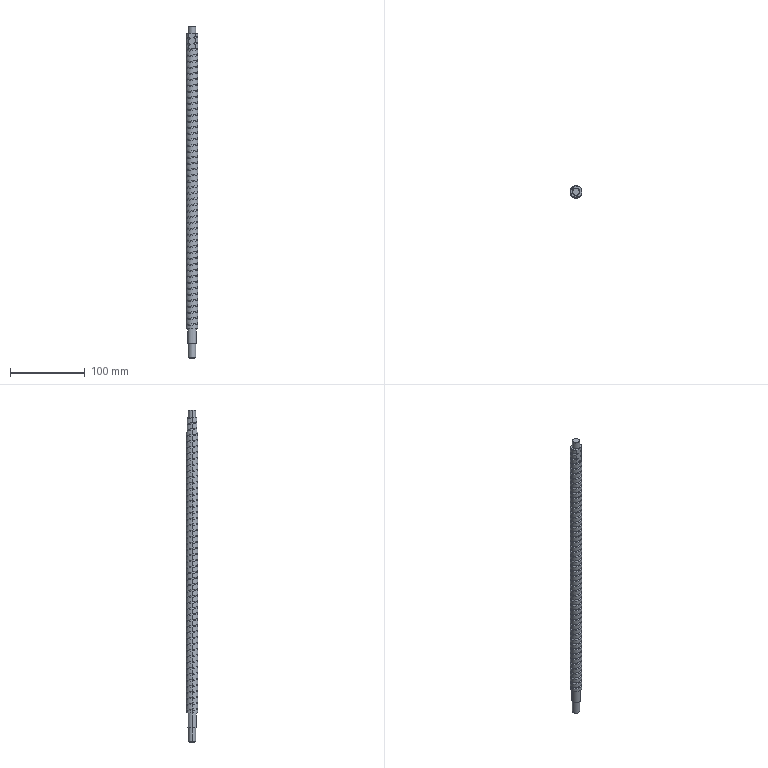Part | STEP file | Ball screw assembly SFUR1604-445 | 1 solid | 136 faces | box 16 x 16 x 445 mm | volume 80049 mm3 | cylinder 114 | plane 12 | spline 6 | cone 4 | commonest cylinder face diameters 16 x104 3 x4 10 x4 12 x2